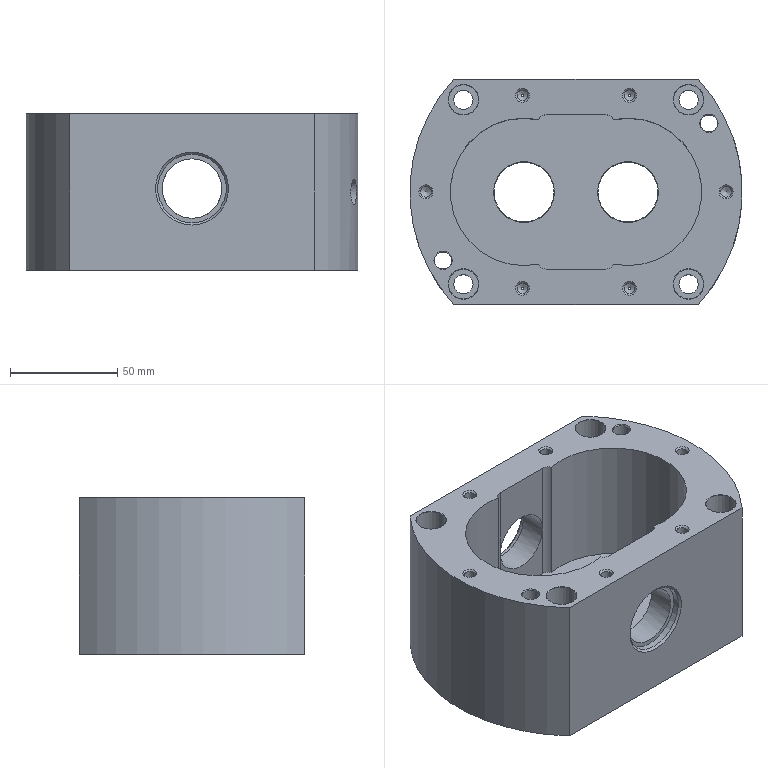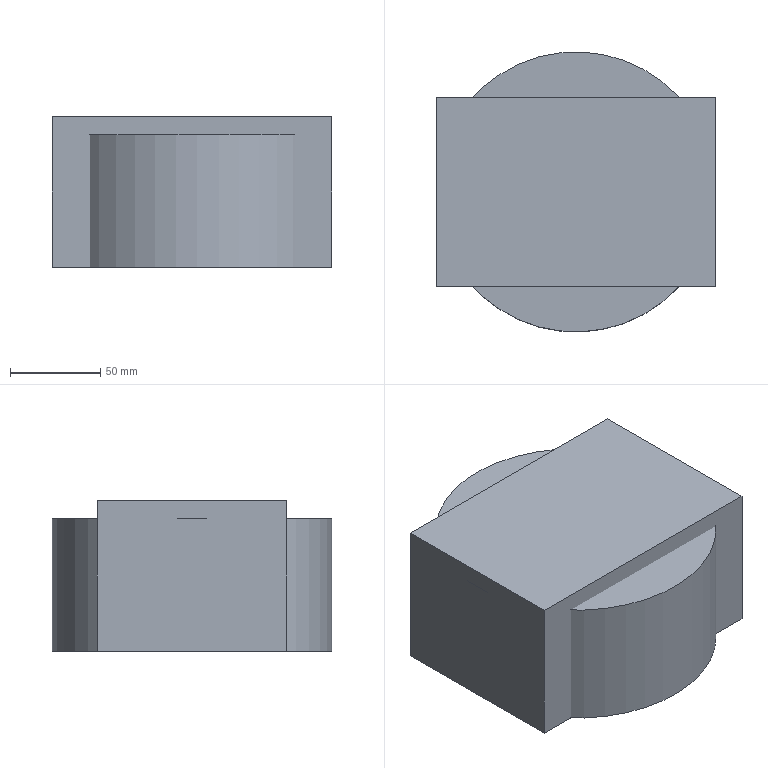CAM job | NX | 3+2 milling, drilling | part box 155 x 105 x 73.2 mm | stock box 155 x 155 x 83.2 mm
Tools:
number,name,description,diameter,corner_radius,flute_length,length,flutes
2,D50,Milling Tool-5 Parameters,50.0,0.0,50.0,75.0,2
10,D10,Milling Tool-5 Parameters,10.0,0.0,50.0,75.0,2
11,D10JING,Milling Tool-5 Parameters,10.0,0.0,50.0,75.0,2
7,D6A45,Milling Tool-5 Parameters,6.0,0.0,50.0,75.0,2
1,ZXZ,Milling Tool-5 Parameters,6.0,0.0,50.0,75.0,2
9,9.0ZT,Drilling Tool,9.0,0.0,35.0,50.0,2
19,7.8ZT,Drilling Tool,7.8,0.0,35.0,50.0,2
17,8.0JD,Milling Tool-5 Parameters,8.0,0.0,30.0,30.0,4
15,5.0ZT,Drilling Tool,5.0,0.0,35.0,50.0,2
14,M6,Milling Tool-5 Parameters,4.2,0.0,30.0,30.0,4
6,D6,Milling Tool-5 Parameters,6.0,0.0,50.0,75.0,2
8,D8,Milling Tool-5 Parameters,8.0,0.0,50.0,75.0,2
16,D6JING,Milling Tool-5 Parameters,6.0,0.0,50.0,75.0,2
23,D6_EXTENDED,Milling Tool-5 Parameters,6.0,0.0,50.0,75.0,2
5,D25R0.5,Milling Tool-5 Parameters,25.0,0.5,50.0,75.0,2
12,D12,Milling Tool-5 Parameters,12.0,0.0,50.0,75.0,2
24,D68.8JD,Milling Tool-5 Parameters,68.8,0.0,30.0,30.0,4
Operations:
program,operation,operation_type,tool,method,geometry_group,spindle_rpm,surface_speed,feed_per_tooth,feed_cut,feed_plunge,cut_length_mm,path_length_mm,cut_time_min,machine_time_min
1,FLOOR_WALL,VolumeBased25DMillingOperation,D50,METHOD,A,1200.0,188.0,0.8333,2000.0,1000.0,38419.403,56366.38,19.426,21.22
1,FLOOR_WALL_COPY,VolumeBased25DMillingOperation,D50,METHOD,A,2500.0,392.0,0.2,1000.0,1000.0,637.25,741.25,0.6372,0.6476
1,HOLE_MILLING,CylinderMilling,D10,METHOD,A,3000.0,94.0,0.3667,2200.0,100.0,2018.245,2131.745,0.9174,0.9287
1,HOLE_MILLING_COPY,CylinderMilling,D10,METHOD,A,3000.0,94.0,0.3667,2200.0,100.0,2155.304,2285.804,0.9797,0.9927
1,HOLE_MILLING_COPY_1,CylinderMilling,D10JING,METHOD,A,5000.0,157.0,0.1,1000.0,100.0,95.013,213.013,0.095,0.1068
1,HOLE_MILLING_COPY_1_COPY,CylinderMilling,D10JING,METHOD,A,5000.0,157.0,0.1,1000.0,100.0,83.88,227.881,0.0839,0.0983
1,PLANAR_MILL,PlanarMilling,D6A45,METHOD,A,7500.0,141.0,0.0833,1250.0,100.0,205.162,312.162,0.1641,0.1748
1,PLANAR_MILL_COPY,PlanarMilling,D6A45,METHOD,A,7500.0,141.0,0.0833,1250.0,100.0,247.927,543.327,0.1983,0.2279
2,DRILLING,Operation,ZXZ,METHOD,B,5000.0,94.0,0.025,250.0,0.0,64.0,636.629,0.256,0.3133
2,DRILLING_COPY,Operation,9.0ZT,METHOD,B,2000.0,56.0,0.0375,150.0,0.0,292.416,930.979,1.949,2.013
2,DRILLING_COPY_COPY,Operation,7.8ZT,METHOD,B,2000.0,56.0,0.0375,150.0,0.0,160.087,522.748,1.067,1.103
2,DRILLING_COPY_COPY_COPY,Operation,8.0JD,METHOD,B,800.0,20.0,0.0125,40.0,0.0,153.4,509.374,3.835,3.871
2,DRILLING_COPY_COPY_1,Operation,5.0ZT,METHOD,B,2000.0,56.0,0.0375,150.0,0.0,104.017,499.434,0.6934,0.733
2,DRILLING_COPY_2_COPY_COPY_1_COPY,Operation,M6,METHOD,B,200.0,3.0,0.0009,1.0,0.0,93.923,479.245,93.923,93.961
2,HOLE_MILLING_COPY_COPY,CylinderMilling,D10,METHOD,B,3000.0,94.0,0.3667,2200.0,100.0,7405.455,7592.955,3.366,3.385
2,HOLE_MILLING_COPY_COPY_COPY,CylinderMilling,D10,METHOD,B,3000.0,94.0,0.3667,2200.0,100.0,3011.056,3227.556,1.369,1.39
2,FLOOR_WALL_1,VolumeBased25DMillingOperation,D10,METHOD,B,3000.0,94.0,0.3667,2200.0,1000.0,25554.852,32590.427,13.51,14.213
2,ZLEVEL_PROFILE_COPY,ZLevelMilling,D6,METHOD,B,5000.0,94.0,0.16,1600.0,1000.0,22826.296,66121.209,15.852,20.182
2,FLOOR_WALL_2,VolumeBased25DMillingOperation,D6JING,METHOD,B,5000.0,157.0,0.1,1000.0,100.0,4685.975,4988.284,4.686,4.716
2,ZLEVEL_PROFILE_COPY_COPY,ZLevelMilling,D6_EXTENDED,METHOD,B,4500.0,84.0,0.1333,1200.0,1000.0,220736.083,223137.274,183.998,184.238
2,PLANAR_MILL_COPY_1,PlanarMilling,D6A45,METHOD,B,7500.0,141.0,0.0833,1250.0,100.0,647.469,1330.933,0.518,0.5863
2,PLANAR_MILL_COPY_1_COPY,PlanarMilling,D6A45,METHOD,B,7500.0,141.0,0.0833,1250.0,100.0,718.257,1587.959,0.5746,0.6616
2,PLANAR_MILL_COPY_1_COPY_COPY,PlanarMilling,D6A45,METHOD,B,7500.0,141.0,0.0833,1250.0,100.0,182.623,387.148,0.1461,0.1666
2,TOOL_OFFSET11,CylinderMilling,D10JING,METHOD,B,5000.0,157.0,0.1,1000.0,100.0,190.999,403.896,0.191,0.2123
2,TOOL_OFFSET_6,CylinderMilling,D6JING,METHOD,B,5000.0,157.0,0.1,1000.0,100.0,206.511,431.011,0.2065,0.229
3,FLOOR_WALL_COPY_1,VolumeBased25DMillingOperation,D50,METHOD,C,1200.0,188.0,0.8333,2000.0,1000.0,29492.913,33715.836,14.834,15.256
3,FLOOR_WALL_COPY_COPY,VolumeBased25DMillingOperation,D50,METHOD,C,2500.0,392.0,0.2,1000.0,1000.0,1016.997,1070.997,1.017,1.022
3,DRILLING_COPY_1,Operation,ZXZ,METHOD,C,5000.0,94.0,0.025,250.0,0.0,24.0,414.311,0.096,0.135
3,DRILLING_COPY_1_COPY,Operation,5.0ZT,METHOD,C,2000.0,42.0,0.05,200.0,0.0,165.013,696.337,0.8251,0.8782
3,DRILLING_COPY_2_COPY_COPY,Operation,M6,METHOD,C,200.0,4.0,0.0016,1.0,0.0,157.442,681.195,157.442,157.494
3,FLOOR_WALL_1_1,VolumeBased25DMillingOperation,D25R0.5,METHOD,C,2000.0,157.0,0.55,2200.0,1000.0,77471.571,82646.618,41.843,42.36
3,ZLEVEL_PROFILE_COPY_COPY_1,ZLevelMilling,D8,METHOD,C,3740.0,94.0,0.2139,1600.0,1000.0,24678.028,43229.009,17.477,19.332
3,FLOOR_WALL_1_COPY_COPY,VolumeBased25DMillingOperation,D12,METHOD,C,4000.0,150.0,0.125,1000.0,500.0,1298.238,1472.638,1.303,1.321
3,ZLEVEL_PROFILE,ZLevelMilling,D12,METHOD,C,5000.0,157.0,0.125,1250.0,100.0,368.482,864.812,0.2948,0.3444
3,HOLE_MILLING_COPY_COPY_COPY_COPY,CylinderMilling,D10,METHOD,C,3000.0,94.0,0.3667,2200.0,100.0,6801.491,7434.491,3.092,3.155
3,HOLE_MILLING_COPY_COPY_COPY_COPY_COPY,CylinderMilling,D10JING,METHOD,C,5000.0,157.0,0.11,1100.0,100.0,4948.537,6697.537,4.499,4.674
3,PLANAR_MILL_COPY_1_COPY_1,PlanarMilling,D6A45,METHOD,C,7500.0,141.0,0.0833,1250.0,100.0,726.606,1833.349,0.5813,0.692
3,DRILLING_1,Operation,D68.8JD,METHOD,C,300.0,94.0,0.0417,50.0,0.0,126.4,364.393,2.528,2.552